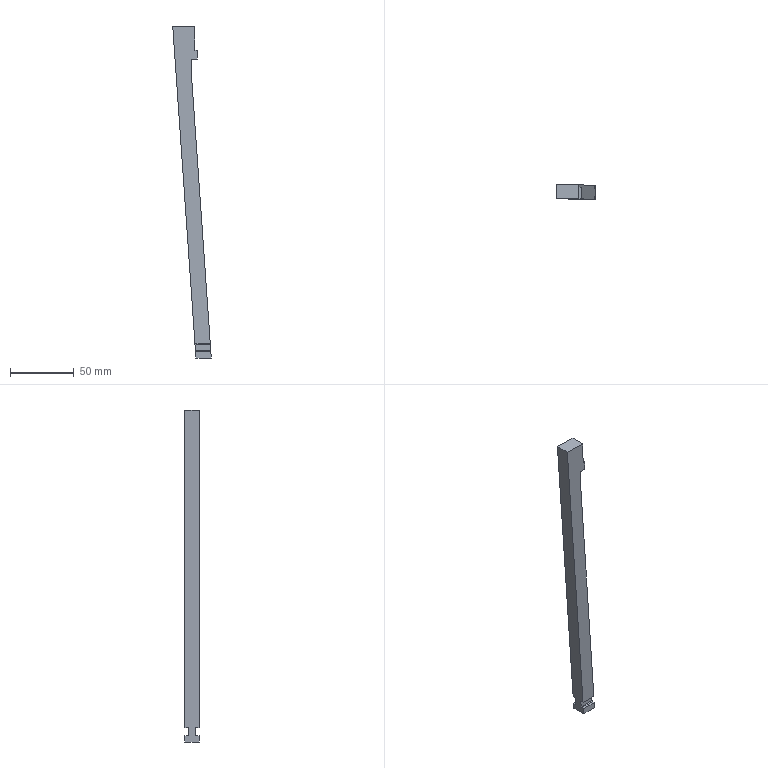Part | Creo | 1 solid | 121 faces | box 30.246 x 11 x 260.516 mm | volume 35454 mm3 | other 79 | plane 36 | cylinder 6 | commonest cylinder face diameters 1 x4 1.865 x1 29.408 x1